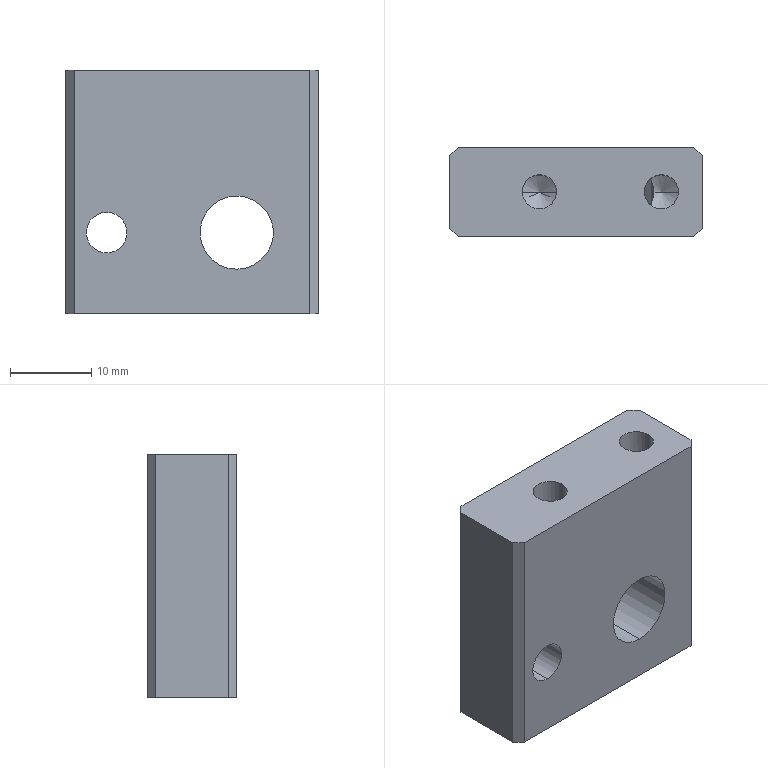Part | STEP file | 1 solid | 22 faces | box 31 x 11 x 30 mm | volume 8762 mm3 | plane 10 | cylinder 8 | cone 4 | commonest cylinder face diameters 4.2 x4 5 x2 9 x2